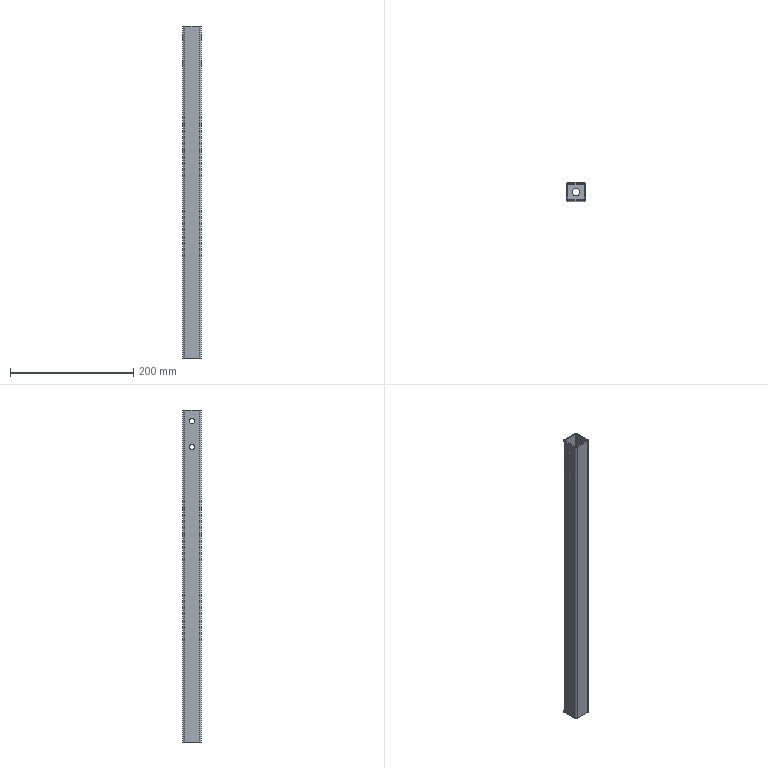Part | STEP file | Leg 30x30x2 | 1 solid | 24 faces | box 30 x 30 x 538 mm | volume 122015 mm3 | cylinder 13 | plane 11 | commonest cylinder face diameters 2 x4 6 x4 8.2 x4 12 x1